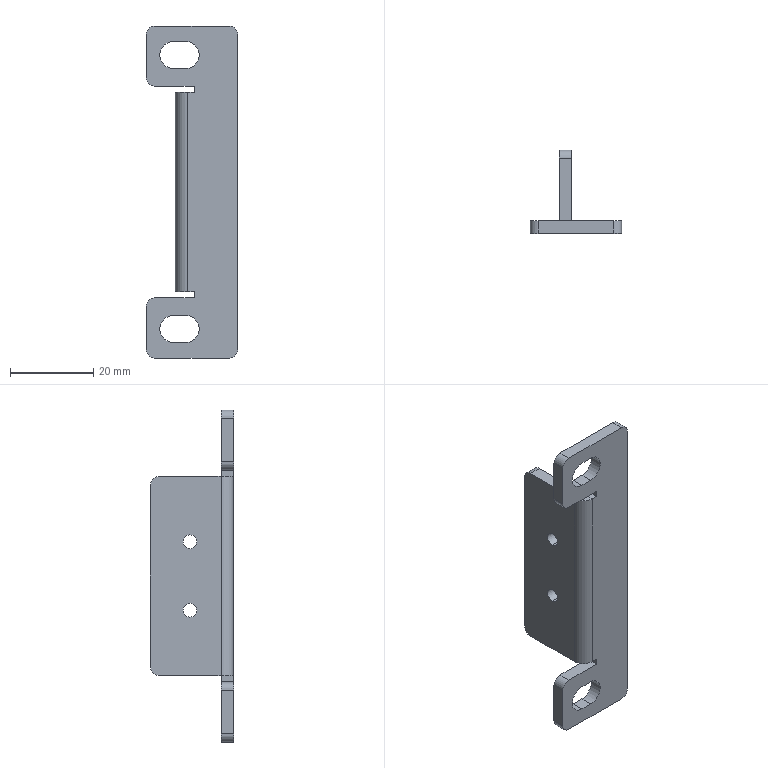Part | STEP file | 1 solid | 42 faces | box 22 x 20 x 80 mm | volume 6135 mm3 | plane 24 | cylinder 18 | commonest cylinder face diameters 4 x8 3.3 x4 6.5 x4 0.02 x1 6.02 x1